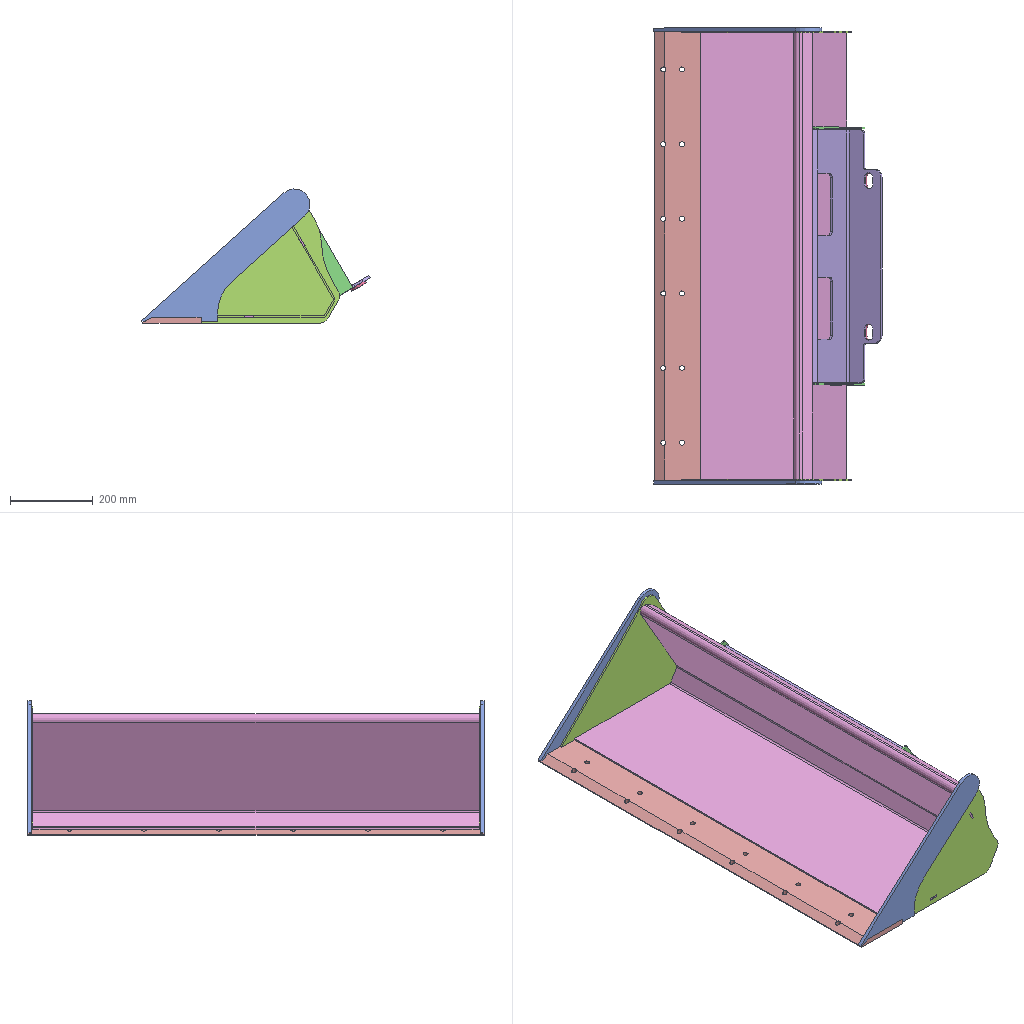Assembly | SolidWorks | 9 different items | 14 placed | box 550 x 1100 x 323 mm
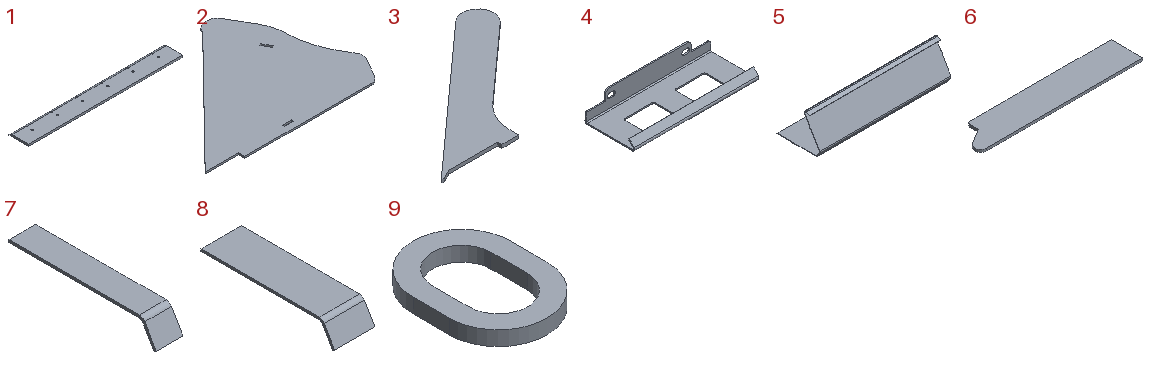Parts list (item | quantity | size | volume | features):
1 | x1 | 1100 x 140 x 14 mm | 1986347 mm3 | features Chamfer 1, FlatPattern 1, SMBaseFlange 1, SheetMetal 1
2 | x2 | 409.722 x 310 x 4 mm | 283862 mm3 | features FlatPattern 1, SMBaseFlange 1, SheetMetal 1
3 | x2 | 405.176 x 319.37 x 8 mm | 281277 mm3 | features FlatPattern 1, SMBaseFlange 1, SheetMetal 1
4 | x1 | 610 x 243.695 x 98.004 mm | 1127789 mm3 | features SM3dBend 2, FlatPattern 1, SMBaseFlange 1, SheetMetal 1
5 | x1 | 1084 x 353.006 x 279.006 mm | 2939163 mm3 | features SM3dBend 3, FlatPattern 1, SMBaseFlange 1, SheetMetal 1
6 | x2 | 255 x 50 x 4 mm | 47889 mm3 | features FlatPattern 1, SMBaseFlange 1, SheetMetal 1
7 | x1 | 60 x 332 x 54.962 mm | 128647 mm3 | features FlatPattern 1, SMBaseFlange 1, SheetMetal 1
8 | x2 | 100 x 332 x 54.962 mm | 214412 mm3 | features FlatPattern 1, SMBaseFlange 1, SheetMetal 1
9 | x2 | 40 x 55 x 6 mm | 6265 mm3 | features FlatPattern 1, SMBaseFlange 1, SheetMetal 1
Mates (type | each side: item.copy, entity, surface, feature):
Coincident | 1.1 face plane Base-Flange1 | 3.1 face plane Base-Flange1 | 3 times
Coincident | 1.1 face plane Base-Flange1 | 3.2 face plane Base-Flange1 | 3 times
Coincident | 1.1 face plane Base-Flange1 | 2.1 face plane Base-Flange1 | 2 times
Coincident | 3.1 face plane Base-Flange1 | 2.1 face plane Base-Flange1
Coincident | 3.2 face plane Base-Flange1 | 2.2 face plane Base-Flange1
Coincident | 1.1 face plane Base-Flange1 | 2.2 face plane Base-Flange1 | 2 times
Coincident | 1.1 face plane Base-Flange1 | 5.1 face plane Base-Flange1
Coincident | 2.1 face plane Base-Flange1 | 5.1 face plane Base-Flange1
DistanceDim | 5.1 face plane Base-Flange1 | 1.1 face plane Base-Flange1
Coincident | 5.1 face plane Base-Flange1 | 8.1 face plane Base-Flange1 | 2 times
DistanceDim | 8.1 face plane Base-Flange1 | 3.1 face plane Base-Flange1
Coincident | 5.1 face plane Base-Flange1 | 8.2 face plane Base-Flange1 | 2 times
DistanceDim | 8.2 face plane Base-Flange1 | 8.1 face plane Base-Flange1
Coincident | 5.1 face plane Base-Flange1 | 7.1 face plane Base-Flange1 | 2 times
DistanceDim | 7.1 face plane Base-Flange1 | 8.1 face plane Base-Flange1
Coincident | 5.1 face plane Base-Flange1 | 4.1 face plane Base-Flange1
Coincident | 5.1 edge | 4.1 face plane Base-Flange1
Coincident | 8.1 face plane Base-Flange1 | 6.1 face plane Base-Flange1
Coincident | 5.1 face plane Base-Flange1 | 6.1 face plane Base-Flange1
Coincident | 8.1 edge | 6.1 face plane Base-Flange1
DistanceDim | 4.1 face plane Base-Flange1 | 6.1 face plane Base-Flange1
Coincident | 5.1 face plane Base-Flange1 | 6.2 face plane Base-Flange1
Coincident | 8.2 face plane Base-Flange1 | 6.2 face plane Base-Flange1
Coincident | 8.2 edge | 6.2 face plane Base-Flange1
Coincident | 4.1 face plane Base-Flange1 | 9.1 face plane Base-Flange1 | 2 times
Concentric | 4.1 face cylinder Base-Flange1 | 9.1 face cylinder Base-Flange1
Coincident | 4.1 face plane Base-Flange1 | 9.2 face plane Base-Flange1 | 2 times
Concentric | 4.1 face cylinder Base-Flange1 | 9.2 face cylinder Base-Flange1